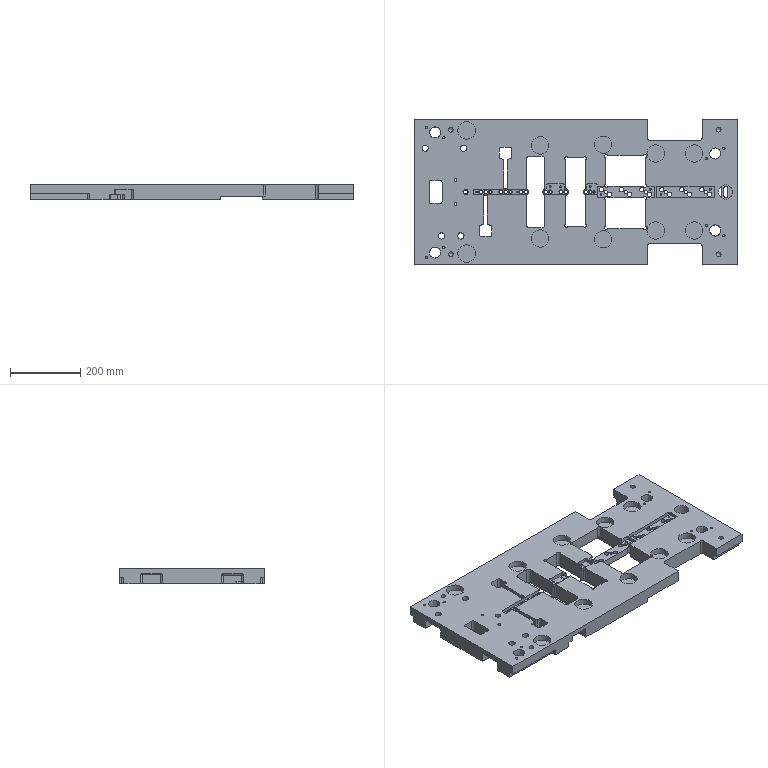Part | STEP file | 1_id130_x_t | 1 solid | 470 faces | box 925 x 416 x 45.006 mm | volume 11838970 mm3 | cylinder 235 | plane 192 | cone 21 | other 16 | spline 6 | commonest cylinder face diameters 6 x39 10 x34 8 x16 12 x16 9.525 x12 13 x12